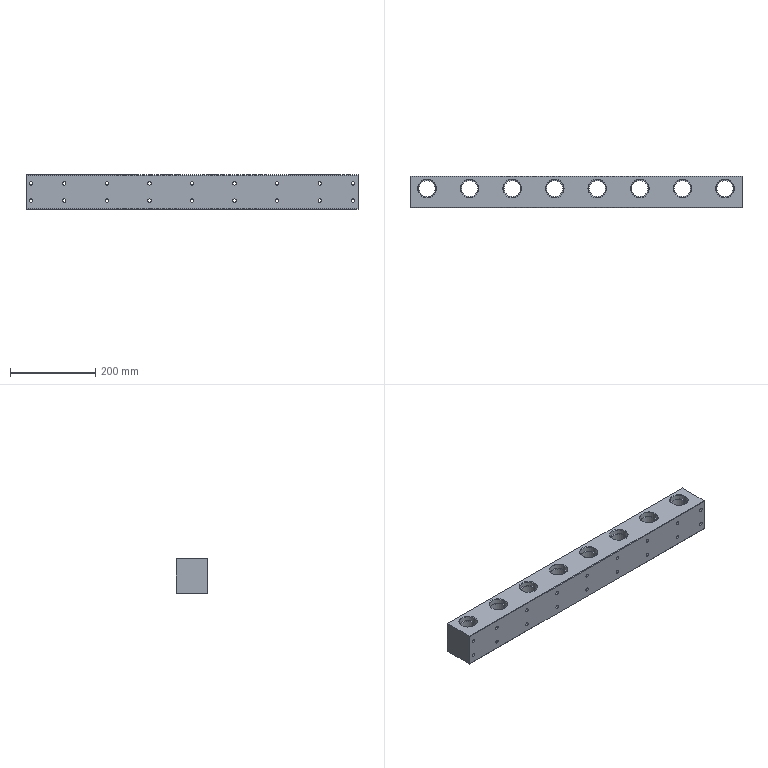Part | SolidWorks | features MirrorPattern 4, HoleWzd 3, LPattern 3, Chamfer 2, ICE 2, Extrusion 1 | 1 solid | 210 faces | box 780 x 74 x 80 mm | volume 3762730 mm3 | cylinder 136 | plane 42 | cone 32 | commonest cylinder face diameters 8 x36 12 x36 42 x32 6.8 x16 38 x16